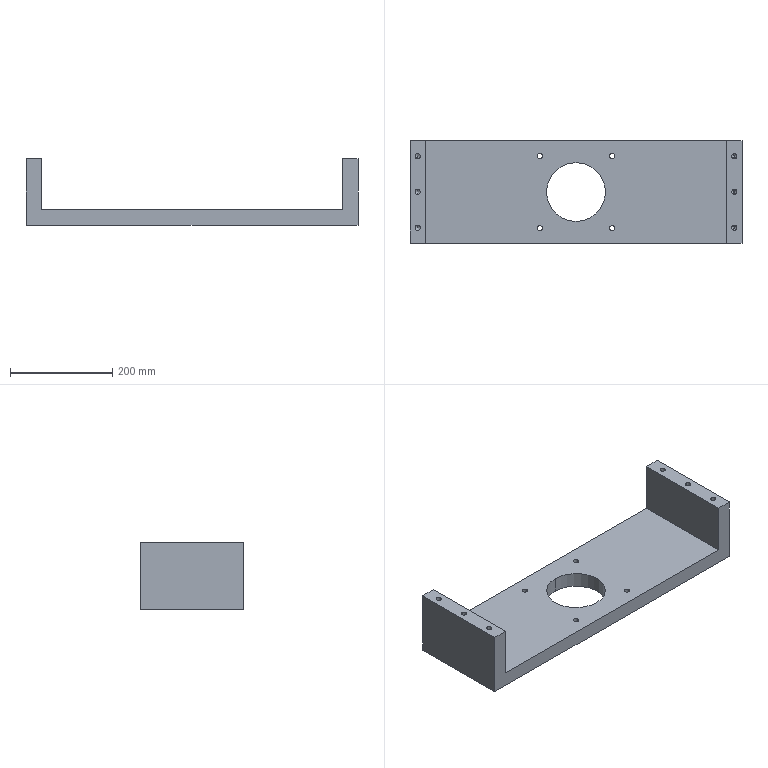Part | SolidWorks | features 3DProfileFeature 1, BaseBody 1, HoleWzd 1, SketchPattern 1 | 1 solid | 44 faces | box 650 x 200 x 130 mm | volume 4762030 mm3 | cylinder 22 | cone 12 | plane 10 | commonest cylinder face diameters 10.2 x20 115 x2
STEP:
#1=CARTESIAN_POINT('',(-65.611,-70.711,15.));
#2=VERTEX_POINT('',#1);
#3=CARTESIAN_POINT('',(-75.811,-70.711,15.));
#4=VERTEX_POINT('',#3);
#5=CARTESIAN_POINT('',(-70.711,-70.711,15.));
#6=DIRECTION('',(0.,0.,-1.));
#7=DIRECTION('',(-1.,0.,0.));
#8=AXIS2_PLACEMENT_3D('',#5,#6,#7);
#9=CIRCLE('',#8,5.1);
#10=EDGE_CURVE('',#2,#4,#9,.T.);
#11=ORIENTED_EDGE('',*,*,#10,.F.);
#12=CARTESIAN_POINT('',(-65.611,-70.711,-15.));
#13=VERTEX_POINT('',#12);
#14=CARTESIAN_POINT('',(-65.611,-70.711,-15.));
#15=DIRECTION('',(0.,0.,-1.));
#16=VECTOR('',#15,1000.);
#17=LINE('',#14,#16);
#18=EDGE_CURVE('',#2,#13,#17,.T.);
#19=ORIENTED_EDGE('',*,*,#18,.T.);
#20=CARTESIAN_POINT('',(-75.811,-70.711,-15.));
#21=VERTEX_POINT('',#20);
#22=CARTESIAN_POINT('',(-70.711,-70.711,-15.));
#23=DIRECTION('',(0.,0.,-1.));
#24=DIRECTION('',(-1.,0.,0.));
#25=AXIS2_PLACEMENT_3D('',#22,#23,#24);
#26=CIRCLE('',#25,5.1);
#27=EDGE_CURVE('',#13,#21,#26,.T.);
#28=ORIENTED_EDGE('',*,*,#27,.T.);
#29=CARTESIAN_POINT('',(-75.811,-70.711,-15.));
#30=DIRECTION('',(0.,0.,-1.));
#31=VECTOR('',#30,1000.);
#32=LINE('',#29,#31);
#33=EDGE_CURVE('',#4,#21,#32,.T.);
#34=ORIENTED_EDGE('',*,*,#33,.F.);
#35=EDGE_LOOP('',(#11,#19,#28,#34));
#36=FACE_OUTER_BOUND('',#35,.T.);
#37=CARTESIAN_POINT('',(-70.711,-70.711,-15.));
#38=DIRECTION('',(0.,0.,-1.));
#39=DIRECTION('',(-1.,0.,0.));
#40=AXIS2_PLACEMENT_3D('',#37,#38,#39);
#41=CYLINDRICAL_SURFACE('',#40,5.1);
#42=ADVANCED_FACE('',(#36),#41,.F.);
#43=CARTESIAN_POINT('',(75.811,-70.711,15.));
#44=VERTEX_POINT('',#43);
#45=CARTESIAN_POINT('',(65.611,-70.711,15.));
#46=VERTEX_POINT('',#45);
#47=CARTESIAN_POINT('',(70.711,-70.711,15.));
#48=DIRECTION('',(0.,0.,-1.));
#49=DIRECTION('',(-1.,0.,0.));
#50=AXIS2_PLACEMENT_3D('',#47,#48,#49);
#51=CIRCLE('',#50,5.1);
#52=EDGE_CURVE('',#44,#46,#51,.T.);
#53=ORIENTED_EDGE('',*,*,#52,.F.);
#54=CARTESIAN_POINT('',(75.811,-70.711,-15.));
#55=VERTEX_POINT('',#54);
#56=CARTESIAN_POINT('',(75.811,-70.711,-15.));
#57=DIRECTION('',(0.,0.,-1.));
#58=VECTOR('',#57,1000.);
#59=LINE('',#56,#58);
#60=EDGE_CURVE('',#44,#55,#59,.T.);
#61=ORIENTED_EDGE('',*,*,#60,.T.);
#62=CARTESIAN_POINT('',(65.611,-70.711,-15.));
#63=VERTEX_POINT('',#62);
#64=CARTESIAN_POINT('',(70.711,-70.711,-15.));
#65=DIRECTION('',(0.,0.,-1.));
#66=DIRECTION('',(-1.,0.,0.));
#67=AXIS2_PLACEMENT_3D('',#64,#65,#66);
#68=CIRCLE('',#67,5.1);
#69=EDGE_CURVE('',#55,#63,#68,.T.);
#70=ORIENTED_EDGE('',*,*,#69,.T.);
#71=CARTESIAN_POINT('',(65.611,-70.711,-15.));
#72=DIRECTION('',(0.,0.,-1.));
#73=VECTOR('',#72,1000.);
#74=LINE('',#71,#73);
#75=EDGE_CURVE('',#46,#63,#74,.T.);
#76=ORIENTED_EDGE('',*,*,#75,.F.);
#77=EDGE_LOOP('',(#53,#61,#70,#76));
#78=FACE_OUTER_BOUND('',#77,.T.);
#79=CARTESIAN_POINT('',(70.711,-70.711,-15.));
#80=DIRECTION('',(0.,0.,-1.));
#81=DIRECTION('',(-1.,0.,0.));
#82=AXIS2_PLACEMENT_3D('',#79,#80,#81);
#83=CYLINDRICAL_SURFACE('',#82,5.1);
#84=ADVANCED_FACE('',(#78),#83,.F.);
#85=CARTESIAN_POINT('',(75.811,70.711,15.));
#86=VERTEX_POINT('',#85);
#87=CARTESIAN_POINT('',(65.611,70.711,15.));
#88=VERTEX_POINT('',#87);
#89=CARTESIAN_POINT('',(70.711,70.711,15.));
#90=DIRECTION('',(0.,0.,-1.));
#91=DIRECTION('',(-1.,0.,0.));
#92=AXIS2_PLACEMENT_3D('',#89,#90,#91);
#93=CIRCLE('',#92,5.1);
#94=EDGE_CURVE('',#86,#88,#93,.T.);
#95=ORIENTED_EDGE('',*,*,#94,.F.);
#96=CARTESIAN_POINT('',(75.811,70.711,-15.));
#97=VERTEX_POINT('',#96);
#98=CARTESIAN_POINT('',(75.811,70.711,-15.));
#99=DIRECTION('',(0.,0.,-1.));
#100=VECTOR('',#99,1000.);
#101=LINE('',#98,#100);
#102=EDGE_CURVE('',#86,#97,#101,.T.);
#103=ORIENTED_EDGE('',*,*,#102,.T.);
#104=CARTESIAN_POINT('',(65.611,70.711,-15.));
#105=VERTEX_POINT('',#104);
#106=CARTESIAN_POINT('',(70.711,70.711,-15.));
#107=DIRECTION('',(0.,0.,-1.));
#108=DIRECTION('',(-1.,0.,0.));
#109=AXIS2_PLACEMENT_3D('',#106,#107,#108);
#110=CIRCLE('',#109,5.1);
#111=EDGE_CURVE('',#97,#105,#110,.T.);
#112=ORIENTED_EDGE('',*,*,#111,.T.);
#113=CARTESIAN_POINT('',(65.611,70.711,-15.));
#114=DIRECTION('',(0.,0.,-1.));
#115=VECTOR('',#114,1000.);
#116=LINE('',#113,#115);
#117=EDGE_CURVE('',#88,#105,#116,.T.);
#118=ORIENTED_EDGE('',*,*,#117,.F.);
#119=EDGE_LOOP('',(#95,#103,#112,#118));
#120=FACE_OUTER_BOUND('',#119,.T.);
#121=CARTESIAN_POINT('',(70.711,70.711,-15.));
#122=DIRECTION('',(0.,0.,-1.));
#123=DIRECTION('',(-1.,0.,0.));
#124=AXIS2_PLACEMENT_3D('',#121,#122,#123);
#125=CYLINDRICAL_SURFACE('',#124,5.1);
#126=ADVANCED_FACE('',(#120),#125,.F.);
#127=CARTESIAN_POINT('',(-65.611,70.711,15.));
#128=VERTEX_POINT('',#127);
#129=CARTESIAN_POINT('',(-75.811,70.711,15.));
#130=VERTEX_POINT('',#129);
#131=CARTESIAN_POINT('',(-70.711,70.711,15.));
#132=DIRECTION('',(0.,0.,-1.));
#133=DIRECTION('',(-1.,0.,0.));
#134=AXIS2_PLACEMENT_3D('',#131,#132,#133);
#135=CIRCLE('',#134,5.1);
#136=EDGE_CURVE('',#128,#130,#135,.T.);
#137=ORIENTED_EDGE('',*,*,#136,.F.);
#138=CARTESIAN_POINT('',(-65.611,70.711,-15.));
#139=VERTEX_POINT('',#138);
#140=CARTESIAN_POINT('',(-65.611,70.711,-15.));
#141=DIRECTION('',(0.,0.,-1.));
#142=VECTOR('',#141,1000.);
#143=LINE('',#140,#142);
#144=EDGE_CURVE('',#128,#139,#143,.T.);
#145=ORIENTED_EDGE('',*,*,#144,.T.);
#146=CARTESIAN_POINT('',(-75.811,70.711,-15.));
#147=VERTEX_POINT('',#146);
#148=CARTESIAN_POINT('',(-70.711,70.711,-15.));
#149=DIRECTION('',(0.,0.,-1.));
#150=DIRECTION('',(-1.,0.,0.));
#151=AXIS2_PLACEMENT_3D('',#148,#149,#150);
#152=CIRCLE('',#151,5.1);
#153=EDGE_CURVE('',#139,#147,#152,.T.);
#154=ORIENTED_EDGE('',*,*,#153,.T.);
#155=CARTESIAN_POINT('',(-75.811,70.711,-15.));
#156=DIRECTION('',(0.,0.,-1.));
#157=VECTOR('',#156,1000.);
#158=LINE('',#155,#157);
#159=EDGE_CURVE('',#130,#147,#158,.T.);
#160=ORIENTED_EDGE('',*,*,#159,.F.);
#161=EDGE_LOOP('',(#137,#145,#154,#160));
#162=FACE_OUTER_BOUND('',#161,.T.);
#163=CARTESIAN_POINT('',(-70.711,70.711,-15.));
#164=DIRECTION('',(0.,0.,-1.));
#165=DIRECTION('',(-1.,0.,0.));
#166=AXIS2_PLACEMENT_3D('',#163,#164,#165);
#167=CYLINDRICAL_SURFACE('',#166,5.1);
#168=ADVANCED_FACE('',(#162),#167,.F.);
#169=CARTESIAN_POINT('',(-310.,64.9,82.25));
#170=VERTEX_POINT('',#169);
#171=CARTESIAN_POINT('',(-310.,75.1,82.25));
#172=VERTEX_POINT('',#171);
#173=CARTESIAN_POINT('',(-310.,70.,82.25));
#174=DIRECTION('',(0.,0.,-1.));
#175=DIRECTION('',(1.,0.,0.));
#176=AXIS2_PLACEMENT_3D('',#173,#174,#175);
#177=CIRCLE('',#176,5.1);
#178=EDGE_CURVE('',#170,#172,#177,.T.);
#179=ORIENTED_EDGE('',*,*,#178,.T.);
#180=CARTESIAN_POINT('',(-310.,75.1,115.));
#181=VERTEX_POINT('',#180);
#182=CARTESIAN_POINT('',(-310.,75.1,82.25));
#183=DIRECTION('',(0.,0.,1.));
#184=VECTOR('',#183,1000.);
#185=LINE('',#182,#184);
#186=EDGE_CURVE('',#172,#181,#185,.T.);
#187=ORIENTED_EDGE('',*,*,#186,.T.);
#188=CARTESIAN_POINT('',(-310.,64.9,115.));
#189=VERTEX_POINT('',#188);
#190=CARTESIAN_POINT('',(-310.,70.,115.));
#191=DIRECTION('',(0.,0.,1.));
#192=DIRECTION('',(0.,-1.,0.));
#193=AXIS2_PLACEMENT_3D('',#190,#191,#192);
#194=CIRCLE('',#193,5.1);
#195=EDGE_CURVE('',#181,#189,#194,.T.);
#196=ORIENTED_EDGE('',*,*,#195,.T.);
#197=CARTESIAN_POINT('',(-310.,64.9,82.25));
#198=DIRECTION('',(0.,0.,1.));
#199=VECTOR('',#198,1000.);
#200=LINE('',#197,#199);
#201=EDGE_CURVE('',#170,#189,#200,.T.);
#202=ORIENTED_EDGE('',*,*,#201,.F.);
#203=EDGE_LOOP('',(#179,#187,#196,#202));
#204=FACE_OUTER_BOUND('',#203,.T.);
#205=CARTESIAN_POINT('',(-310.,70.,82.25));
#206=DIRECTION('',(0.,0.,1.));
#207=DIRECTION('',(0.,-1.,0.));
#208=AXIS2_PLACEMENT_3D('',#205,#206,#207);
#209=CYLINDRICAL_SURFACE('',#208,5.1);
#210=ADVANCED_FACE('',(#204),#209,.F.);
#211=CARTESIAN_POINT('',(-310.,70.,79.186));
#212=VERTEX_POINT('',#211);
#213=CARTESIAN_POINT('',(-310.,70.,79.186));
#214=DIRECTION('',(0.,-0.8572,0.515));
#215=VECTOR('',#214,1000.);
#216=LINE('',#213,#215);
#217=EDGE_CURVE('',#212,#170,#216,.T.);
#218=ORIENTED_EDGE('',*,*,#217,.F.);
#219=CARTESIAN_POINT('',(-310.,70.,79.186));
#220=DIRECTION('',(0.,0.8572,0.515));
#221=VECTOR('',#220,1000.);
#222=LINE('',#219,#221);
#223=EDGE_CURVE('',#212,#172,#222,.T.);
#224=ORIENTED_EDGE('',*,*,#223,.T.);
#225=ORIENTED_EDGE('',*,*,#178,.F.);
#226=EDGE_LOOP('',(#218,#224,#225));
#227=FACE_OUTER_BOUND('',#226,.T.);
#228=CARTESIAN_POINT('',(-310.,70.,1079.186));
#229=DIRECTION('',(0.,0.,1.));
#230=DIRECTION('',(0.,-1.,0.));
#231=AXIS2_PLACEMENT_3D('',#228,#229,#230);
#232=CONICAL_SURFACE('',#231,1664.279,1.03);
#233=ADVANCED_FACE('',(#227),#232,.F.);
#234=CARTESIAN_POINT('',(-310.,-75.1,82.25));
#235=VERTEX_POINT('',#234);
#236=CARTESIAN_POINT('',(-310.,-64.9,82.25));
#237=VERTEX_POINT('',#236);
#238=CARTESIAN_POINT('',(-310.,-70.,82.25));
#239=DIRECTION('',(0.,0.,-1.));
#240=DIRECTION('',(1.,0.,0.));
#241=AXIS2_PLACEMENT_3D('',#238,#239,#240);
#242=CIRCLE('',#241,5.1);
#243=EDGE_CURVE('',#235,#237,#242,.T.);
#244=ORIENTED_EDGE('',*,*,#243,.T.);
#245=CARTESIAN_POINT('',(-310.,-64.9,115.));
#246=VERTEX_POINT('',#245);
#247=CARTESIAN_POINT('',(-310.,-64.9,82.25));
#248=DIRECTION('',(0.,0.,1.));
#249=VECTOR('',#248,1000.);
#250=LINE('',#247,#249);
#251=EDGE_CURVE('',#237,#246,#250,.T.);
#252=ORIENTED_EDGE('',*,*,#251,.T.);
#253=CARTESIAN_POINT('',(-310.,-75.1,115.));
#254=VERTEX_POINT('',#253);
#255=CARTESIAN_POINT('',(-310.,-70.,115.));
#256=DIRECTION('',(0.,0.,-1.));
#257=DIRECTION('',(0.,-1.,0.));
#258=AXIS2_PLACEMENT_3D('',#255,#256,#257);
#259=CIRCLE('',#258,5.1);
#260=EDGE_CURVE('',#254,#246,#259,.T.);
#261=ORIENTED_EDGE('',*,*,#260,.F.);
#262=CARTESIAN_POINT('',(-310.,-75.1,82.25));
#263=DIRECTION('',(0.,0.,1.));
#264=VECTOR('',#263,1000.);
#265=LINE('',#262,#264);
#266=EDGE_CURVE('',#235,#254,#265,.T.);
#267=ORIENTED_EDGE('',*,*,#266,.F.);
#268=EDGE_LOOP('',(#244,#252,#261,#267));
#269=FACE_OUTER_BOUND('',#268,.T.);
#270=CARTESIAN_POINT('',(-310.,-70.,82.25));
#271=DIRECTION('',(0.,0.,1.));
#272=DIRECTION('',(0.,-1.,0.));
#273=AXIS2_PLACEMENT_3D('',#270,#271,#272);
#274=CYLINDRICAL_SURFACE('',#273,5.1);
#275=ADVANCED_FACE('',(#269),#274,.F.);
#276=CARTESIAN_POINT('',(-310.,-5.1,82.25));
#277=VERTEX_POINT('',#276);
#278=CARTESIAN_POINT('',(-310.,5.1,82.25));
#279=VERTEX_POINT('',#278);
#280=CARTESIAN_POINT('',(-310.,0.,82.25));
#281=DIRECTION('',(0.,0.,-1.));
#282=DIRECTION('',(1.,0.,0.));
#283=AXIS2_PLACEMENT_3D('',#280,#281,#282);
#284=CIRCLE('',#283,5.1);
#285=EDGE_CURVE('',#277,#279,#284,.T.);
#286=ORIENTED_EDGE('',*,*,#285,.T.);
#287=CARTESIAN_POINT('',(-310.,5.1,115.));
#288=VERTEX_POINT('',#287);
#289=CARTESIAN_POINT('',(-310.,5.1,82.25));
#290=DIRECTION('',(0.,0.,1.));
#291=VECTOR('',#290,1000.);
#292=LINE('',#289,#291);
#293=EDGE_CURVE('',#279,#288,#292,.T.);
#294=ORIENTED_EDGE('',*,*,#293,.T.);
#295=CARTESIAN_POINT('',(-310.,-5.1,115.));
#296=VERTEX_POINT('',#295);
#297=CARTESIAN_POINT('',(-310.,0.,115.));
#298=DIRECTION('',(0.,0.,-1.));
#299=DIRECTION('',(0.,-1.,0.));
#300=AXIS2_PLACEMENT_3D('',#297,#298,#299);
#301=CIRCLE('',#300,5.1);
#302=EDGE_CURVE('',#296,#288,#301,.T.);
#303=ORIENTED_EDGE('',*,*,#302,.F.);
#304=CARTESIAN_POINT('',(-310.,-5.1,82.25));
#305=DIRECTION('',(0.,0.,1.));
#306=VECTOR('',#305,1000.);
#307=LINE('',#304,#306);
#308=EDGE_CURVE('',#277,#296,#307,.T.);
#309=ORIENTED_EDGE('',*,*,#308,.F.);
#310=EDGE_LOOP('',(#286,#294,#303,#309));
#311=FACE_OUTER_BOUND('',#310,.T.);
#312=CARTESIAN_POINT('',(-310.,0.,82.25));
#313=DIRECTION('',(0.,0.,1.));
#314=DIRECTION('',(0.,-1.,0.));
#315=AXIS2_PLACEMENT_3D('',#312,#313,#314);
#316=CYLINDRICAL_SURFACE('',#315,5.1);
#317=ADVANCED_FACE('',(#311),#316,.F.);
#318=CARTESIAN_POINT('',(-310.,-70.,79.186));
#319=VERTEX_POINT('',#318);
#320=CARTESIAN_POINT('',(-310.,-70.,79.186));
#321=DIRECTION('',(0.,-0.8572,0.515));
#322=VECTOR('',#321,1000.);
#323=LINE('',#320,#322);
#324=EDGE_CURVE('',#319,#235,#323,.T.);
#325=ORIENTED_EDGE('',*,*,#324,.F.);
#326=CARTESIAN_POINT('',(-310.,-70.,79.186));
#327=DIRECTION('',(0.,0.8572,0.515));
#328=VECTOR('',#327,1000.);
#329=LINE('',#326,#328);
#330=EDGE_CURVE('',#319,#237,#329,.T.);
#331=ORIENTED_EDGE('',*,*,#330,.T.);
#332=ORIENTED_EDGE('',*,*,#243,.F.);
#333=EDGE_LOOP('',(#325,#331,#332));
#334=FACE_OUTER_BOUND('',#333,.T.);
#335=CARTESIAN_POINT('',(-310.,-70.,1079.186));
#336=DIRECTION('',(0.,0.,1.));
#337=DIRECTION('',(0.,-1.,0.));
#338=AXIS2_PLACEMENT_3D('',#335,#336,#337);
#339=CONICAL_SURFACE('',#338,1664.279,1.03);
#340=ADVANCED_FACE('',(#334),#339,.F.);
#341=CARTESIAN_POINT('',(-310.,0.,79.186));
#342=VERTEX_POINT('',#341);
#343=CARTESIAN_POINT('',(-310.,0.,79.186));
#344=DIRECTION('',(0.,-0.8572,0.515));
#345=VECTOR('',#344,1000.);
#346=LINE('',#343,#345);
#347=EDGE_CURVE('',#342,#277,#346,.T.);
#348=ORIENTED_EDGE('',*,*,#347,.F.);
#349=CARTESIAN_POINT('',(-310.,0.,79.186));
#350=DIRECTION('',(0.,0.8572,0.515));
#351=VECTOR('',#350,1000.);
#352=LINE('',#349,#351);
#353=EDGE_CURVE('',#342,#279,#352,.T.);
#354=ORIENTED_EDGE('',*,*,#353,.T.);
#355=ORIENTED_EDGE('',*,*,#285,.F.);
#356=EDGE_LOOP('',(#348,#354,#355));
#357=FACE_OUTER_BOUND('',#356,.T.);
#358=CARTESIAN_POINT('',(-310.,0.,1079.186));
#359=DIRECTION('',(0.,0.,1.));
#360=DIRECTION('',(0.,-1.,0.));
#361=AXIS2_PLACEMENT_3D('',#358,#359,#360);
#362=CONICAL_SURFACE('',#361,1664.279,1.03);
#363=ADVANCED_FACE('',(#357),#362,.F.);
#364=CARTESIAN_POINT('',(0.,57.5,-15.));
#365=VERTEX_POINT('',#364);
#366=CARTESIAN_POINT('',(0.,-57.5,-15.));
#367=VERTEX_POINT('',#366);
#368=CARTESIAN_POINT('',(0.,0.,-15.));
#369=DIRECTION('',(0.,0.,1.));
#370=DIRECTION('',(0.,-1.,0.));
#371=AXIS2_PLACEMENT_3D('',#368,#369,#370);
#372=CIRCLE('',#371,57.5);
#373=EDGE_CURVE('',#365,#367,#372,.T.);
#374=ORIENTED_EDGE('',*,*,#373,.F.);
#375=CARTESIAN_POINT('',(0.,57.5,15.));
#376=VERTEX_POINT('',#375);
#377=CARTESIAN_POINT('',(0.,57.5,-15.));
#378=DIRECTION('',(0.,0.,1.));
#379=VECTOR('',#378,1000.);
#380=LINE('',#377,#379);
#381=EDGE_CURVE('',#365,#376,#380,.T.);
#382=ORIENTED_EDGE('',*,*,#381,.T.);
#383=CARTESIAN_POINT('',(0.,-57.5,15.));
#384=VERTEX_POINT('',#383);
#385=CARTESIAN_POINT('',(0.,0.,15.));
#386=DIRECTION('',(0.,0.,1.));
#387=DIRECTION('',(0.,-1.,0.));
#388=AXIS2_PLACEMENT_3D('',#385,#386,#387);
#389=CIRCLE('',#388,57.5);
#390=EDGE_CURVE('',#376,#384,#389,.T.);
#391=ORIENTED_EDGE('',*,*,#390,.T.);
#392=CARTESIAN_POINT('',(0.,-57.5,-15.));
#393=DIRECTION('',(0.,0.,1.));
#394=VECTOR('',#393,1000.);
#395=LINE('',#392,#394);
#396=EDGE_CURVE('',#367,#384,#395,.T.);
#397=ORIENTED_EDGE('',*,*,#396,.F.);
#398=EDGE_LOOP('',(#374,#382,#391,#397));
#399=FACE_OUTER_BOUND('',#398,.T.);
#400=CARTESIAN_POINT('',(0.,0.,-15.));
#401=DIRECTION('',(0.,0.,1.));
#402=DIRECTION('',(0.,-1.,0.));
#403=AXIS2_PLACEMENT_3D('',#400,#401,#402);
#404=CYLINDRICAL_SURFACE('',#403,57.5);
#405=ADVANCED_FACE('',(#399),#404,.F.);
#406=CARTESIAN_POINT('',(310.,64.9,82.25));
#407=VERTEX_POINT('',#406);
#408=CARTESIAN_POINT('',(310.,75.1,82.25));
#409=VERTEX_POINT('',#408);
#410=CARTESIAN_POINT('',(310.,70.,82.25));
#411=DIRECTION('',(0.,0.,-1.));
#412=DIRECTION('',(1.,0.,0.));
#413=AXIS2_PLACEMENT_3D('',#410,#411,#412);
#414=CIRCLE('',#413,5.1);
#415=EDGE_CURVE('',#407,#409,#414,.T.);
#416=ORIENTED_EDGE('',*,*,#415,.T.);
#417=CARTESIAN_POINT('',(310.,75.1,115.));
#418=VERTEX_POINT('',#417);
#419=CARTESIAN_POINT('',(310.,75.1,82.25));
#420=DIRECTION('',(0.,0.,1.));
#421=VECTOR('',#420,1000.);
#422=LINE('',#419,#421);
#423=EDGE_CURVE('',#409,#418,#422,.T.);
#424=ORIENTED_EDGE('',*,*,#423,.T.);
#425=CARTESIAN_POINT('',(310.,64.9,115.));
#426=VERTEX_POINT('',#425);
#427=CARTESIAN_POINT('',(310.,70.,115.));
#428=DIRECTION('',(0.,0.,-1.));
#429=DIRECTION('',(0.,-1.,0.));
#430=AXIS2_PLACEMENT_3D('',#427,#428,#429);
#431=CIRCLE('',#430,5.1);
#432=EDGE_CURVE('',#426,#418,#431,.T.);
#433=ORIENTED_EDGE('',*,*,#432,.F.);
#434=CARTESIAN_POINT('',(310.,64.9,82.25));
#435=DIRECTION('',(0.,0.,1.));
#436=VECTOR('',#435,1000.);
#437=LINE('',#434,#436);
#438=EDGE_CURVE('',#407,#426,#437,.T.);
#439=ORIENTED_EDGE('',*,*,#438,.F.);
#440=EDGE_LOOP('',(#416,#424,#433,#439));
#441=FACE_OUTER_BOUND('',#440,.T.);
#442=CARTESIAN_POINT('',(310.,70.,82.25));
#443=DIRECTION('',(0.,0.,1.));
#444=DIRECTION('',(0.,-1.,0.));
#445=AXIS2_PLACEMENT_3D('',#442,#443,#444);
#446=CYLINDRICAL_SURFACE('',#445,5.1);
#447=ADVANCED_FACE('',(#441),#446,.F.);
#448=CARTESIAN_POINT('',(310.,-5.1,82.25));
#449=VERTEX_POINT('',#448);
#450=CARTESIAN_POINT('',(310.,5.1,82.25));
#451=VERTEX_POINT('',#450);
#452=CARTESIAN_POINT('',(310.,0.,82.25));
#453=DIRECTION('',(0.,0.,-1.));
#454=DIRECTION('',(1.,0.,0.));
#455=AXIS2_PLACEMENT_3D('',#452,#453,#454);
#456=CIRCLE('',#455,5.1);
#457=EDGE_CURVE('',#449,#451,#456,.T.);
#458=ORIENTED_EDGE('',*,*,#457,.T.);
#459=CARTESIAN_POINT('',(310.,5.1,115.));
#460=VERTEX_POINT('',#459);
#461=CARTESIAN_POINT('',(310.,5.1,82.25));
#462=DIRECTION('',(0.,0.,1.));
#463=VECTOR('',#462,1000.);
#464=LINE('',#461,#463);
#465=EDGE_CURVE('',#451,#460,#464,.T.);
#466=ORIENTED_EDGE('',*,*,#465,.T.);
#467=CARTESIAN_POINT('',(310.,-5.1,115.));
#468=VERTEX_POINT('',#467);
#469=CARTESIAN_POINT('',(310.,0.,115.));
#470=DIRECTION('',(0.,0.,-1.));
#471=DIRECTION('',(0.,-1.,0.));
#472=AXIS2_PLACEMENT_3D('',#469,#470,#471);
#473=CIRCLE('',#472,5.1);
#474=EDGE_CURVE('',#468,#460,#473,.T.);
#475=ORIENTED_EDGE('',*,*,#474,.F.);
#476=CARTESIAN_POINT('',(310.,-5.1,82.25));
#477=DIRECTION('',(0.,0.,1.));
#478=VECTOR('',#477,1000.);
#479=LINE('',#476,#478);
#480=EDGE_CURVE('',#449,#468,#479,.T.);
#481=ORIENTED_EDGE('',*,*,#480,.F.);
#482=EDGE_LOOP('',(#458,#466,#475,#481));
#483=FACE_OUTER_BOUND('',#482,.T.);
#484=CARTESIAN_POINT('',(310.,0.,82.25));
#485=DIRECTION('',(0.,0.,1.));
#486=DIRECTION('',(0.,-1.,0.));
#487=AXIS2_PLACEMENT_3D('',#484,#485,#486);
#488=CYLINDRICAL_SURFACE('',#487,5.1);
#489=ADVANCED_FACE('',(#483),#488,.F.);
#490=CARTESIAN_POINT('',(310.,-75.1,82.25));
#491=VERTEX_POINT('',#490);
#492=CARTESIAN_POINT('',(310.,-64.9,82.25));
#493=VERTEX_POINT('',#492);
#494=CARTESIAN_POINT('',(310.,-70.,82.25));
#495=DIRECTION('',(0.,0.,-1.));
#496=DIRECTION('',(1.,0.,0.));
#497=AXIS2_PLACEMENT_3D('',#494,#495,#496);
#498=CIRCLE('',#497,5.1);
#499=EDGE_CURVE('',#491,#493,#498,.T.);
#500=ORIENTED_EDGE('',*,*,#499,.T.);
#501=CARTESIAN_POINT('',(310.,-64.9,115.));
#502=VERTEX_POINT('',#501);
#503=CARTESIAN_POINT('',(310.,-64.9,82.25));
#504=DIRECTION('',(0.,0.,1.));
#505=VECTOR('',#504,1000.);
#506=LINE('',#503,#505);
#507=EDGE_CURVE('',#493,#502,#506,.T.);
#508=ORIENTED_EDGE('',*,*,#507,.T.);
#509=CARTESIAN_POINT('',(310.,-75.1,115.));
#510=VERTEX_POINT('',#509);
#511=CARTESIAN_POINT('',(310.,-70.,115.));
#512=DIRECTION('',(0.,0.,-1.));
#513=DIRECTION('',(0.,-1.,0.));
#514=AXIS2_PLACEMENT_3D('',#511,#512,#513);
#515=CIRCLE('',#514,5.1);
#516=EDGE_CURVE('',#510,#502,#515,.T.);
#517=ORIENTED_EDGE('',*,*,#516,.F.);
#518=CARTESIAN_POINT('',(310.,-75.1,82.25));
#519=DIRECTION('',(0.,0.,1.));
#520=VECTOR('',#519,1000.);
#521=LINE('',#518,#520);
#522=EDGE_CURVE('',#491,#510,#521,.T.);
#523=ORIENTED_EDGE('',*,*,#522,.F.);
#524=EDGE_LOOP('',(#500,#508,#517,#523));
#525=FACE_OUTER_BOUND('',#524,.T.);
#526=CARTESIAN_POINT('',(310.,-70.,82.25));
#527=DIRECTION('',(0.,0.,1.));
#528=DIRECTION('',(0.,-1.,0.));
#529=AXIS2_PLACEMENT_3D('',#526,#527,#528);
#530=CYLINDRICAL_SURFACE('',#529,5.1);
#531=ADVANCED_FACE('',(#525),#530,.F.);
#532=CARTESIAN_POINT('',(310.,70.,79.186));
#533=VERTEX_POINT('',#532);
#534=CARTESIAN_POINT('',(310.,70.,79.186));
#535=DIRECTION('',(0.,-0.8572,0.515));
#536=VECTOR('',#535,1000.);
#537=LINE('',#534,#536);
#538=EDGE_CURVE('',#533,#407,#537,.T.);
#539=ORIENTED_EDGE('',*,*,#538,.F.);
#540=CARTESIAN_POINT('',(310.,70.,79.186));
#541=DIRECTION('',(0.,0.8572,0.515));
#542=VECTOR('',#541,1000.);
#543=LINE('',#540,#542);
#544=EDGE_CURVE('',#533,#409,#543,.T.);
#545=ORIENTED_EDGE('',*,*,#544,.T.);
#546=ORIENTED_EDGE('',*,*,#415,.F.);
#547=EDGE_LOOP('',(#539,#545,#546));
#548=FACE_OUTER_BOUND('',#547,.T.);
#549=CARTESIAN_POINT('',(310.,70.,1079.186));
#550=DIRECTION('',(0.,0.,1.));
#551=DIRECTION('',(0.,-1.,0.));
#552=AXIS2_PLACEMENT_3D('',#549,#550,#551);
#553=CONICAL_SURFACE('',#552,1664.279,1.03);
#554=ADVANCED_FACE('',(#548),#553,.F.);
#555=CARTESIAN_POINT('',(310.,0.,79.186));
#556=VERTEX_POINT('',#555);
#557=CARTESIAN_POINT('',(310.,0.,79.186));
#558=DIRECTION('',(0.,-0.8572,0.515));
#559=VECTOR('',#558,1000.);
#560=LINE('',#557,#559);
#561=EDGE_CURVE('',#556,#449,#560,.T.);
#562=ORIENTED_EDGE('',*,*,#561,.F.);
#563=CARTESIAN_POINT('',(310.,0.,79.186));
#564=DIRECTION('',(0.,0.8572,0.515));
#565=VECTOR('',#564,1000.);
#566=LINE('',#563,#565);
#567=EDGE_CURVE('',#556,#451,#566,.T.);
#568=ORIENTED_EDGE('',*,*,#567,.T.);
#569=ORIENTED_EDGE('',*,*,#457,.F.);
#570=EDGE_LOOP('',(#562,#568,#569));
#571=FACE_OUTER_BOUND('',#570,.T.);
#572=CARTESIAN_POINT('',(310.,0.,1079.186));
#573=DIRECTION('',(0.,0.,1.));
#574=DIRECTION('',(0.,-1.,0.));
#575=AXIS2_PLACEMENT_3D('',#572,#573,#574);
#576=CONICAL_SURFACE('',#575,1664.279,1.03);
#577=ADVANCED_FACE('',(#571),#576,.F.);
#578=CARTESIAN_POINT('',(310.,-70.,79.186));
#579=VERTEX_POINT('',#578);
#580=CARTESIAN_POINT('',(310.,-70.,79.186));
#581=DIRECTION('',(0.,-0.8572,0.515));
#582=VECTOR('',#581,1000.);
#583=LINE('',#580,#582);
#584=EDGE_CURVE('',#579,#491,#583,.T.);
#585=ORIENTED_EDGE('',*,*,#584,.F.);
#586=CARTESIAN_POINT('',(310.,-70.,79.186));
#587=DIRECTION('',(0.,0.8572,0.515));
#588=VECTOR('',#587,1000.);
#589=LINE('',#586,#588);
#590=EDGE_CURVE('',#579,#493,#589,.T.);
#591=ORIENTED_EDGE('',*,*,#590,.T.);
#592=ORIENTED_EDGE('',*,*,#499,.F.);
#593=EDGE_LOOP('',(#585,#591,#592));
#594=FACE_OUTER_BOUND('',#593,.T.);
#595=CARTESIAN_POINT('',(310.,-70.,1079.186));
#596=DIRECTION('',(0.,0.,1.));
#597=DIRECTION('',(0.,-1.,0.));
#598=AXIS2_PLACEMENT_3D('',#595,#596,#597);
#599=CONICAL_SURFACE('',#598,1664.279,1.03);
#600=ADVANCED_FACE('',(#594),#599,.F.);
#601=ORIENTED_EDGE('',*,*,#186,.F.);
#602=CARTESIAN_POINT('',(-310.,70.,82.25));
#603=DIRECTION('',(0.,0.,-1.));
#604=DIRECTION('',(1.,0.,0.));
#605=AXIS2_PLACEMENT_3D('',#602,#603,#604);
#606=CIRCLE('',#605,5.1);
#607=EDGE_CURVE('',#172,#170,#606,.T.);
#608=ORIENTED_EDGE('',*,*,#607,.T.);
#609=ORIENTED_EDGE('',*,*,#201,.T.);
#610=CARTESIAN_POINT('',(-310.,70.,115.));
#611=DIRECTION('',(0.,0.,1.));
#612=DIRECTION('',(0.,-1.,0.));
#613=AXIS2_PLACEMENT_3D('',#610,#611,#612);
#614=CIRCLE('',#613,5.1);
#615=EDGE_CURVE('',#189,#181,#614,.T.);
#616=ORIENTED_EDGE('',*,*,#615,.T.);
#617=EDGE_LOOP('',(#601,#608,#609,#616));
#618=FACE_OUTER_BOUND('',#617,.T.);
#619=CARTESIAN_POINT('',(-310.,70.,82.25));
#620=DIRECTION('',(0.,0.,1.));
#621=DIRECTION('',(0.,-1.,0.));
#622=AXIS2_PLACEMENT_3D('',#619,#620,#621);
#623=CYLINDRICAL_SURFACE('',#622,5.1);
#624=ADVANCED_FACE('',(#618),#623,.F.);
#625=ORIENTED_EDGE('',*,*,#260,.T.);
#626=CARTESIAN_POINT('',(-310.,-70.,115.));
#627=DIRECTION('',(0.,0.,-1.));
#628=DIRECTION('',(0.,-1.,0.));
#629=AXIS2_PLACEMENT_3D('',#626,#627,#628);
#630=CIRCLE('',#629,5.1);
#631=EDGE_CURVE('',#246,#254,#630,.T.);
#632=ORIENTED_EDGE('',*,*,#631,.T.);
#633=EDGE_LOOP('',(#625,#632));
#634=FACE_BOUND('',#633,.T.);
#635=ORIENTED_EDGE('',*,*,#302,.T.);
#636=CARTESIAN_POINT('',(-310.,0.,115.));
#637=DIRECTION('',(0.,0.,-1.));
#638=DIRECTION('',(0.,-1.,0.));
#639=AXIS2_PLACEMENT_3D('',#636,#637,#638);
#640=CIRCLE('',#639,5.1);
#641=EDGE_CURVE('',#288,#296,#640,.T.);
#642=ORIENTED_EDGE('',*,*,#641,.T.);
#643=EDGE_LOOP('',(#635,#642));
#644=FACE_BOUND('',#643,.T.);
#645=ORIENTED_EDGE('',*,*,#615,.F.);
#646=ORIENTED_EDGE('',*,*,#195,.F.);
#647=EDGE_LOOP('',(#645,#646));
#648=FACE_BOUND('',#647,.T.);
#649=CARTESIAN_POINT('',(-295.,-100.,115.));
#650=VERTEX_POINT('',#649);
#651=CARTESIAN_POINT('',(-295.,100.,115.));
#652=VERTEX_POINT('',#651);
#653=CARTESIAN_POINT('',(-295.,0.,115.));
#654=DIRECTION('',(0.,1.,0.));
#655=VECTOR('',#654,1000.);
#656=LINE('',#653,#655);
#657=EDGE_CURVE('',#650,#652,#656,.T.);
#658=ORIENTED_EDGE('',*,*,#657,.T.);
#659=CARTESIAN_POINT('',(-325.,100.,115.));
#660=VERTEX_POINT('',#659);
#661=CARTESIAN_POINT('',(-310.,100.,115.));
#662=DIRECTION('',(-1.,0.,0.));
#663=VECTOR('',#662,1000.);
#664=LINE('',#661,#663);
#665=EDGE_CURVE('',#652,#660,#664,.T.);
#666=ORIENTED_EDGE('',*,*,#665,.T.);
#667=CARTESIAN_POINT('',(-325.,-100.,115.));
#668=VERTEX_POINT('',#667);
#669=CARTESIAN_POINT('',(-325.,0.,115.));
#670=DIRECTION('',(0.,-1.,0.));
#671=VECTOR('',#670,1000.);
#672=LINE('',#669,#671);
#673=EDGE_CURVE('',#660,#668,#672,.T.);
#674=ORIENTED_EDGE('',*,*,#673,.T.);
#675=CARTESIAN_POINT('',(-310.,-100.,115.));
#676=DIRECTION('',(1.,0.,0.));
#677=VECTOR('',#676,1000.);
#678=LINE('',#675,#677);
#679=EDGE_CURVE('',#668,#650,#678,.T.);
#680=ORIENTED_EDGE('',*,*,#679,.T.);
#681=EDGE_LOOP('',(#658,#666,#674,#680));
#682=FACE_OUTER_BOUND('',#681,.T.);
#683=CARTESIAN_POINT('',(-325.,-100.,115.));
#684=DIRECTION('',(0.,0.,1.));
#685=DIRECTION('',(1.,0.,0.));
#686=AXIS2_PLACEMENT_3D('',#683,#684,#685);
#687=PLANE('',#686);
#688=ADVANCED_FACE('',(#634,#644,#648,#682),#687,.T.);
#689=ORIENTED_EDGE('',*,*,#223,.F.);
#690=ORIENTED_EDGE('',*,*,#217,.T.);
#691=ORIENTED_EDGE('',*,*,#607,.F.);
#692=EDGE_LOOP('',(#689,#690,#691));
#693=FACE_OUTER_BOUND('',#692,.T.);
#694=CARTESIAN_POINT('',(-310.,70.,1079.186));
#695=DIRECTION('',(0.,0.,1.));
#696=DIRECTION('',(0.,-1.,0.));
#697=AXIS2_PLACEMENT_3D('',#694,#695,#696);
#698=CONICAL_SURFACE('',#697,1664.279,1.03);
#699=ADVANCED_FACE('',(#693),#698,.F.);
#700=ORIENTED_EDGE('',*,*,#251,.F.);
#701=CARTESIAN_POINT('',(-310.,-70.,82.25));
#702=DIRECTION('',(0.,0.,-1.));
#703=DIRECTION('',(1.,0.,0.));
#704=AXIS2_PLACEMENT_3D('',#701,#702,#703);
#705=CIRCLE('',#704,5.1);
#706=EDGE_CURVE('',#237,#235,#705,.T.);
#707=ORIENTED_EDGE('',*,*,#706,.T.);
#708=ORIENTED_EDGE('',*,*,#266,.T.);
#709=ORIENTED_EDGE('',*,*,#631,.F.);
#710=EDGE_LOOP('',(#700,#707,#708,#709));
#711=FACE_OUTER_BOUND('',#710,.T.);
#712=CARTESIAN_POINT('',(-310.,-70.,82.25));
#713=DIRECTION('',(0.,0.,1.));
#714=DIRECTION('',(0.,-1.,0.));
#715=AXIS2_PLACEMENT_3D('',#712,#713,#714);
#716=CYLINDRICAL_SURFACE('',#715,5.1);
#717=ADVANCED_FACE('',(#711),#716,.F.);
#718=ORIENTED_EDGE('',*,*,#293,.F.);
#719=CARTESIAN_POINT('',(-310.,0.,82.25));
#720=DIRECTION('',(0.,0.,-1.));
#721=DIRECTION('',(1.,0.,0.));
#722=AXIS2_PLACEMENT_3D('',#719,#720,#721);
#723=CIRCLE('',#722,5.1);
#724=EDGE_CURVE('',#279,#277,#723,.T.);
#725=ORIENTED_EDGE('',*,*,#724,.T.);
#726=ORIENTED_EDGE('',*,*,#308,.T.);
#727=ORIENTED_EDGE('',*,*,#641,.F.);
#728=EDGE_LOOP('',(#718,#725,#726,#727));
#729=FACE_OUTER_BOUND('',#728,.T.);
#730=CARTESIAN_POINT('',(-310.,0.,82.25));
#731=DIRECTION('',(0.,0.,1.));
#732=DIRECTION('',(0.,-1.,0.));
#733=AXIS2_PLACEMENT_3D('',#730,#731,#732);
#734=CYLINDRICAL_SURFACE('',#733,5.1);
#735=ADVANCED_FACE('',(#729),#734,.F.);
#736=CARTESIAN_POINT('',(-325.,100.,-15.));
#737=VERTEX_POINT('',#736);
#738=CARTESIAN_POINT('',(-325.,100.,50.));
#739=DIRECTION('',(0.,0.,-1.));
#740=VECTOR('',#739,1000.);
#741=LINE('',#738,#740);
#742=EDGE_CURVE('',#660,#737,#741,.T.);
#743=ORIENTED_EDGE('',*,*,#742,.F.);
#744=ORIENTED_EDGE('',*,*,#665,.F.);
#745=CARTESIAN_POINT('',(-295.,100.,15.));
#746=VERTEX_POINT('',#745);
#747=CARTESIAN_POINT('',(-295.,100.,50.));
#748=DIRECTION('',(0.,0.,1.));
#749=VECTOR('',#748,1000.);
#750=LINE('',#747,#749);
#751=EDGE_CURVE('',#746,#652,#750,.T.);
#752=ORIENTED_EDGE('',*,*,#751,.F.);
#753=CARTESIAN_POINT('',(295.,100.,15.));
#754=VERTEX_POINT('',#753);
#755=CARTESIAN_POINT('',(0.,100.,15.));
#756=DIRECTION('',(-1.,0.,0.));
#757=VECTOR('',#756,1000.);
#758=LINE('',#755,#757);
#759=EDGE_CURVE('',#754,#746,#758,.T.);
#760=ORIENTED_EDGE('',*,*,#759,.F.);
#761=CARTESIAN_POINT('',(295.,100.,115.));
#762=VERTEX_POINT('',#761);
#763=CARTESIAN_POINT('',(295.,100.,50.));
#764=DIRECTION('',(0.,0.,-1.));
#765=VECTOR('',#764,1000.);
#766=LINE('',#763,#765);
#767=EDGE_CURVE('',#762,#754,#766,.T.);
#768=ORIENTED_EDGE('',*,*,#767,.F.);
#769=CARTESIAN_POINT('',(325.,100.,115.));
#770=VERTEX_POINT('',#769);
#771=CARTESIAN_POINT('',(0.,100.,115.));
#772=DIRECTION('',(-1.,0.,0.));
#773=VECTOR('',#772,1000.);
#774=LINE('',#771,#773);
#775=EDGE_CURVE('',#770,#762,#774,.T.);
#776=ORIENTED_EDGE('',*,*,#775,.F.);
#777=CARTESIAN_POINT('',(325.,100.,-15.));
#778=VERTEX_POINT('',#777);
#779=CARTESIAN_POINT('',(325.,100.,50.));
#780=DIRECTION('',(0.,0.,1.));
#781=VECTOR('',#780,1000.);
#782=LINE('',#779,#781);
#783=EDGE_CURVE('',#778,#770,#782,.T.);
#784=ORIENTED_EDGE('',*,*,#783,.F.);
#785=CARTESIAN_POINT('',(0.,100.,-15.));
#786=DIRECTION('',(1.,0.,0.));
#787=VECTOR('',#786,1000.);
#788=LINE('',#785,#787);
#789=EDGE_CURVE('',#737,#778,#788,.T.);
#790=ORIENTED_EDGE('',*,*,#789,.F.);
#791=EDGE_LOOP('',(#743,#744,#752,#760,#768,#776,#784,#790));
#792=FACE_OUTER_BOUND('',#791,.T.);
#793=CARTESIAN_POINT('',(-325.,100.,115.));
#794=DIRECTION('',(0.,-1.,0.));
#795=DIRECTION('',(0.,0.,-1.));
#796=AXIS2_PLACEMENT_3D('',#793,#794,#795);
#797=PLANE('',#796);
#798=ADVANCED_FACE('',(#792),#797,.F.);
#799=ORIENTED_EDGE('',*,*,#751,.T.);
#800=ORIENTED_EDGE('',*,*,#657,.F.);
#801=CARTESIAN_POINT('',(-295.,-100.,15.));
#802=VERTEX_POINT('',#801);
#803=CARTESIAN_POINT('',(-295.,-100.,65.));
#804=DIRECTION('',(0.,0.,1.));
#805=VECTOR('',#804,1000.);
#806=LINE('',#803,#805);
#807=EDGE_CURVE('',#802,#650,#806,.T.);
#808=ORIENTED_EDGE('',*,*,#807,.F.);
#809=CARTESIAN_POINT('',(-295.,0.,15.));
#810=DIRECTION('',(0.,-1.,0.));
#811=VECTOR('',#810,1000.);
#812=LINE('',#809,#811);
#813=EDGE_CURVE('',#746,#802,#812,.T.);
#814=ORIENTED_EDGE('',*,*,#813,.F.);
#815=EDGE_LOOP('',(#799,#800,#808,#814));
#816=FACE_OUTER_BOUND('',#815,.T.);
#817=CARTESIAN_POINT('',(-295.,-100.,15.));
#818=DIRECTION('',(-1.,0.,0.));
#819=DIRECTION('',(0.,0.,1.));
#820=AXIS2_PLACEMENT_3D('',#817,#818,#819);
#821=PLANE('',#820);
#822=ADVANCED_FACE('',(#816),#821,.F.);
#823=CARTESIAN_POINT('',(325.,-100.,115.));
#824=VERTEX_POINT('',#823);
#825=CARTESIAN_POINT('',(325.,-100.,-15.));
#826=VERTEX_POINT('',#825);
#827=CARTESIAN_POINT('',(325.,-100.,50.));
#828=DIRECTION('',(0.,0.,-1.));
#829=VECTOR('',#828,1000.);
#830=LINE('',#827,#829);
#831=EDGE_CURVE('',#824,#826,#830,.T.);
#832=ORIENTED_EDGE('',*,*,#831,.F.);
#833=CARTESIAN_POINT('',(295.,-100.,115.));
#834=VERTEX_POINT('',#833);
#835=CARTESIAN_POINT('',(0.,-100.,115.));
#836=DIRECTION('',(1.,0.,0.));
#837=VECTOR('',#836,1000.);
#838=LINE('',#835,#837);
#839=EDGE_CURVE('',#834,#824,#838,.T.);
#840=ORIENTED_EDGE('',*,*,#839,.F.);
#841=CARTESIAN_POINT('',(295.,-100.,15.));
#842=VERTEX_POINT('',#841);
#843=CARTESIAN_POINT('',(295.,-100.,50.));
#844=DIRECTION('',(0.,0.,1.));
#845=VECTOR('',#844,1000.);
#846=LINE('',#843,#845);
#847=EDGE_CURVE('',#842,#834,#846,.T.);
#848=ORIENTED_EDGE('',*,*,#847,.F.);
#849=CARTESIAN_POINT('',(0.,-100.,15.));
#850=DIRECTION('',(1.,0.,0.));
#851=VECTOR('',#850,1000.);
#852=LINE('',#849,#851);
#853=EDGE_CURVE('',#802,#842,#852,.T.);
#854=ORIENTED_EDGE('',*,*,#853,.F.);
#855=ORIENTED_EDGE('',*,*,#807,.T.);
#856=ORIENTED_EDGE('',*,*,#679,.F.);
#857=CARTESIAN_POINT('',(-325.,-100.,-15.));
#858=VERTEX_POINT('',#857);
#859=CARTESIAN_POINT('',(-325.,-100.,50.));
#860=DIRECTION('',(0.,0.,1.));
#861=VECTOR('',#860,1000.);
#862=LINE('',#859,#861);
#863=EDGE_CURVE('',#858,#668,#862,.T.);
#864=ORIENTED_EDGE('',*,*,#863,.F.);
#865=CARTESIAN_POINT('',(0.,-100.,-15.));
#866=DIRECTION('',(-1.,0.,0.));
#867=VECTOR('',#866,1000.);
#868=LINE('',#865,#867);
#869=EDGE_CURVE('',#826,#858,#868,.T.);
#870=ORIENTED_EDGE('',*,*,#869,.F.);
#871=EDGE_LOOP('',(#832,#840,#848,#854,#855,#856,#864,#870));
#872=FACE_OUTER_BOUND('',#871,.T.);
#873=CARTESIAN_POINT('',(-325.,-100.,-15.));
#874=DIRECTION('',(0.,1.,0.));
#875=DIRECTION('',(0.,0.,1.));
#876=AXIS2_PLACEMENT_3D('',#873,#874,#875);
#877=PLANE('',#876);
#878=ADVANCED_FACE('',(#872),#877,.F.);
#879=ORIENTED_EDGE('',*,*,#863,.T.);
#880=ORIENTED_EDGE('',*,*,#673,.F.);
#881=ORIENTED_EDGE('',*,*,#742,.T.);
#882=CARTESIAN_POINT('',(-325.,0.,-15.));
#883=DIRECTION('',(0.,1.,0.));
#884=VECTOR('',#883,1000.);
#885=LINE('',#882,#884);
#886=EDGE_CURVE('',#858,#737,#885,.T.);
#887=ORIENTED_EDGE('',*,*,#886,.F.);
#888=EDGE_LOOP('',(#879,#880,#881,#887));
#889=FACE_OUTER_BOUND('',#888,.T.);
#890=CARTESIAN_POINT('',(-325.,-100.,115.));
#891=DIRECTION('',(1.,0.,0.));
#892=DIRECTION('',(0.,0.,-1.));
#893=AXIS2_PLACEMENT_3D('',#890,#891,#892);
#894=PLANE('',#893);
#895=ADVANCED_FACE('',(#889),#894,.F.);
#896=ORIENTED_EDGE('',*,*,#330,.F.);
#897=ORIENTED_EDGE('',*,*,#324,.T.);
#898=ORIENTED_EDGE('',*,*,#706,.F.);
#899=EDGE_LOOP('',(#896,#897,#898));
#900=FACE_OUTER_BOUND('',#899,.T.);
#901=CARTESIAN_POINT('',(-310.,-70.,1079.186));
#902=DIRECTION('',(0.,0.,1.));
#903=DIRECTION('',(0.,-1.,0.));
#904=AXIS2_PLACEMENT_3D('',#901,#902,#903);
#905=CONICAL_SURFACE('',#904,1664.279,1.03);
#906=ADVANCED_FACE('',(#900),#905,.F.);
#907=ORIENTED_EDGE('',*,*,#353,.F.);
#908=ORIENTED_EDGE('',*,*,#347,.T.);
#909=ORIENTED_EDGE('',*,*,#724,.F.);
#910=EDGE_LOOP('',(#907,#908,#909));
#911=FACE_OUTER_BOUND('',#910,.T.);
#912=CARTESIAN_POINT('',(-310.,0.,1079.186));
#913=DIRECTION('',(0.,0.,1.));
#914=DIRECTION('',(0.,-1.,0.));
#915=AXIS2_PLACEMENT_3D('',#912,#913,#914);
#916=CONICAL_SURFACE('',#915,1664.279,1.03);
#917=ADVANCED_FACE('',(#911),#916,.F.);
#918=CARTESIAN_POINT('',(-70.711,-70.711,-15.));
#919=DIRECTION('',(0.,0.,-1.));
#920=DIRECTION('',(-1.,0.,0.));
#921=AXIS2_PLACEMENT_3D('',#918,#919,#920);
#922=CIRCLE('',#921,5.1);
#923=EDGE_CURVE('',#21,#13,#922,.T.);
#924=ORIENTED_EDGE('',*,*,#923,.F.);
#925=ORIENTED_EDGE('',*,*,#27,.F.);
#926=EDGE_LOOP('',(#924,#925));
#927=FACE_BOUND('',#926,.T.);
#928=CARTESIAN_POINT('',(70.711,-70.711,-15.));
#929=DIRECTION('',(0.,0.,-1.));
#930=DIRECTION('',(-1.,0.,0.));
#931=AXIS2_PLACEMENT_3D('',#928,#929,#930);
#932=CIRCLE('',#931,5.1);
#933=EDGE_CURVE('',#63,#55,#932,.T.);
#934=ORIENTED_EDGE('',*,*,#933,.F.);
#935=ORIENTED_EDGE('',*,*,#69,.F.);
#936=EDGE_LOOP('',(#934,#935));
#937=FACE_BOUND('',#936,.T.);
#938=CARTESIAN_POINT('',(70.711,70.711,-15.));
#939=DIRECTION('',(0.,0.,-1.));
#940=DIRECTION('',(-1.,0.,0.));
#941=AXIS2_PLACEMENT_3D('',#938,#939,#940);
#942=CIRCLE('',#941,5.1);
#943=EDGE_CURVE('',#105,#97,#942,.T.);
#944=ORIENTED_EDGE('',*,*,#943,.F.);
#945=ORIENTED_EDGE('',*,*,#111,.F.);
#946=EDGE_LOOP('',(#944,#945));
#947=FACE_BOUND('',#946,.T.);
#948=CARTESIAN_POINT('',(-70.711,70.711,-15.));
#949=DIRECTION('',(0.,0.,-1.));
#950=DIRECTION('',(-1.,0.,0.));
#951=AXIS2_PLACEMENT_3D('',#948,#949,#950);
#952=CIRCLE('',#951,5.1);
#953=EDGE_CURVE('',#147,#139,#952,.T.);
#954=ORIENTED_EDGE('',*,*,#953,.F.);
#955=ORIENTED_EDGE('',*,*,#153,.F.);
#956=EDGE_LOOP('',(#954,#955));
#957=FACE_BOUND('',#956,.T.);
#958=CARTESIAN_POINT('',(0.,0.,-15.));
#959=DIRECTION('',(0.,0.,1.));
#960=DIRECTION('',(0.,-1.,0.));
#961=AXIS2_PLACEMENT_3D('',#958,#959,#960);
#962=CIRCLE('',#961,57.5);
#963=EDGE_CURVE('',#367,#365,#962,.T.);
#964=ORIENTED_EDGE('',*,*,#963,.T.);
#965=ORIENTED_EDGE('',*,*,#373,.T.);
#966=EDGE_LOOP('',(#964,#965));
#967=FACE_BOUND('',#966,.T.);
#968=ORIENTED_EDGE('',*,*,#886,.T.);
#969=ORIENTED_EDGE('',*,*,#789,.T.);
#970=CARTESIAN_POINT('',(325.,0.,-15.));
#971=DIRECTION('',(0.,-1.,0.));
#972=VECTOR('',#971,1000.);
#973=LINE('',#970,#972);
#974=EDGE_CURVE('',#778,#826,#973,.T.);
#975=ORIENTED_EDGE('',*,*,#974,.T.);
#976=ORIENTED_EDGE('',*,*,#869,.T.);
#977=EDGE_LOOP('',(#968,#969,#975,#976));
#978=FACE_OUTER_BOUND('',#977,.T.);
#979=CARTESIAN_POINT('',(325.,-100.,-15.));
#980=DIRECTION('',(0.,0.,-1.));
#981=DIRECTION('',(-1.,0.,0.));
#982=AXIS2_PLACEMENT_3D('',#979,#980,#981);
#983=PLANE('',#982);
#984=ADVANCED_FACE('',(#927,#937,#947,#957,#967,#978),#983,.T.);
#985=CARTESIAN_POINT('',(-70.711,-70.711,15.));
#986=DIRECTION('',(0.,0.,-1.));
#987=DIRECTION('',(-1.,0.,0.));
#988=AXIS2_PLACEMENT_3D('',#985,#986,#987);
#989=CIRCLE('',#988,5.1);
#990=EDGE_CURVE('',#4,#2,#989,.T.);
#991=ORIENTED_EDGE('',*,*,#990,.T.);
#992=ORIENTED_EDGE('',*,*,#10,.T.);
#993=EDGE_LOOP('',(#991,#992));
#994=FACE_BOUND('',#993,.T.);
#995=CARTESIAN_POINT('',(70.711,-70.711,15.));
#996=DIRECTION('',(0.,0.,-1.));
#997=DIRECTION('',(-1.,0.,0.));
#998=AXIS2_PLACEMENT_3D('',#995,#996,#997);
#999=CIRCLE('',#998,5.1);
#1000=EDGE_CURVE('',#46,#44,#999,.T.);
#1001=ORIENTED_EDGE('',*,*,#1000,.T.);
#1002=ORIENTED_EDGE('',*,*,#52,.T.);
#1003=EDGE_LOOP('',(#1001,#1002));
#1004=FACE_BOUND('',#1003,.T.);
#1005=CARTESIAN_POINT('',(70.711,70.711,15.));
#1006=DIRECTION('',(0.,0.,-1.));
#1007=DIRECTION('',(-1.,0.,0.));
#1008=AXIS2_PLACEMENT_3D('',#1005,#1006,#1007);
#1009=CIRCLE('',#1008,5.1);
#1010=EDGE_CURVE('',#88,#86,#1009,.T.);
#1011=ORIENTED_EDGE('',*,*,#1010,.T.);
#1012=ORIENTED_EDGE('',*,*,#94,.T.);
#1013=EDGE_LOOP('',(#1011,#1012));
#1014=FACE_BOUND('',#1013,.T.);
#1015=CARTESIAN_POINT('',(-70.711,70.711,15.));
#1016=DIRECTION('',(0.,0.,-1.));
#1017=DIRECTION('',(-1.,0.,0.));
#1018=AXIS2_PLACEMENT_3D('',#1015,#1016,#1017);
#1019=CIRCLE('',#1018,5.1);
#1020=EDGE_CURVE('',#130,#128,#1019,.T.);
#1021=ORIENTED_EDGE('',*,*,#1020,.T.);
#1022=ORIENTED_EDGE('',*,*,#136,.T.);
#1023=EDGE_LOOP('',(#1021,#1022));
#1024=FACE_BOUND('',#1023,.T.);
#1025=CARTESIAN_POINT('',(0.,0.,15.));
#1026=DIRECTION('',(0.,0.,1.));
#1027=DIRECTION('',(0.,-1.,0.));
#1028=AXIS2_PLACEMENT_3D('',#1025,#1026,#1027);
#1029=CIRCLE('',#1028,57.5);
#1030=EDGE_CURVE('',#384,#376,#1029,.T.);
#1031=ORIENTED_EDGE('',*,*,#1030,.F.);
#1032=ORIENTED_EDGE('',*,*,#390,.F.);
#1033=EDGE_LOOP('',(#1031,#1032));
#1034=FACE_BOUND('',#1033,.T.);
#1035=ORIENTED_EDGE('',*,*,#759,.T.);
#1036=ORIENTED_EDGE('',*,*,#813,.T.);
#1037=ORIENTED_EDGE('',*,*,#853,.T.);
#1038=CARTESIAN_POINT('',(295.,0.,15.));
#1039=DIRECTION('',(0.,-1.,0.));
#1040=VECTOR('',#1039,1000.);
#1041=LINE('',#1038,#1040);
#1042=EDGE_CURVE('',#754,#842,#1041,.T.);
#1043=ORIENTED_EDGE('',*,*,#1042,.F.);
#1044=EDGE_LOOP('',(#1035,#1036,#1037,#1043));
#1045=FACE_OUTER_BOUND('',#1044,.T.);
#1046=CARTESIAN_POINT('',(295.,-100.,15.));
#1047=DIRECTION('',(0.,0.,-1.));
#1048=DIRECTION('',(-1.,0.,0.));
#1049=AXIS2_PLACEMENT_3D('',#1046,#1047,#1048);
#1050=PLANE('',#1049);
#1051=ADVANCED_FACE('',(#994,#1004,#1014,#1024,#1034,#1045),#1050,.F.);
#1052=ORIENTED_EDGE('',*,*,#847,.T.);
#1053=CARTESIAN_POINT('',(295.,0.,115.));
#1054=DIRECTION('',(0.,-1.,0.));
#1055=VECTOR('',#1054,1000.);
#1056=LINE('',#1053,#1055);
#1057=EDGE_CURVE('',#762,#834,#1056,.T.);
#1058=ORIENTED_EDGE('',*,*,#1057,.F.);
#1059=ORIENTED_EDGE('',*,*,#767,.T.);
#1060=ORIENTED_EDGE('',*,*,#1042,.T.);
#1061=EDGE_LOOP('',(#1052,#1058,#1059,#1060));
#1062=FACE_OUTER_BOUND('',#1061,.T.);
#1063=CARTESIAN_POINT('',(295.,-100.,115.));
#1064=DIRECTION('',(1.,0.,0.));
#1065=DIRECTION('',(0.,0.,-1.));
#1066=AXIS2_PLACEMENT_3D('',#1063,#1064,#1065);
#1067=PLANE('',#1066);
#1068=ADVANCED_FACE('',(#1062),#1067,.F.);
#1069=ORIENTED_EDGE('',*,*,#432,.T.);
#1070=CARTESIAN_POINT('',(310.,70.,115.));
#1071=DIRECTION('',(0.,0.,-1.));
#1072=DIRECTION('',(0.,-1.,0.));
#1073=AXIS2_PLACEMENT_3D('',#1070,#1071,#1072);
#1074=CIRCLE('',#1073,5.1);
#1075=EDGE_CURVE('',#418,#426,#1074,.T.);
#1076=ORIENTED_EDGE('',*,*,#1075,.T.);
#1077=EDGE_LOOP('',(#1069,#1076));
#1078=FACE_BOUND('',#1077,.T.);
#1079=ORIENTED_EDGE('',*,*,#474,.T.);
#1080=CARTESIAN_POINT('',(310.,0.,115.));
#1081=DIRECTION('',(0.,0.,-1.));
#1082=DIRECTION('',(0.,-1.,0.));
#1083=AXIS2_PLACEMENT_3D('',#1080,#1081,#1082);
#1084=CIRCLE('',#1083,5.1);
#1085=EDGE_CURVE('',#460,#468,#1084,.T.);
#1086=ORIENTED_EDGE('',*,*,#1085,.T.);
#1087=EDGE_LOOP('',(#1079,#1086));
#1088=FACE_BOUND('',#1087,.T.);
#1089=ORIENTED_EDGE('',*,*,#516,.T.);
#1090=CARTESIAN_POINT('',(310.,-70.,115.));
#1091=DIRECTION('',(0.,0.,-1.));
#1092=DIRECTION('',(0.,-1.,0.));
#1093=AXIS2_PLACEMENT_3D('',#1090,#1091,#1092);
#1094=CIRCLE('',#1093,5.1);
#1095=EDGE_CURVE('',#502,#510,#1094,.T.);
#1096=ORIENTED_EDGE('',*,*,#1095,.T.);
#1097=EDGE_LOOP('',(#1089,#1096));
#1098=FACE_BOUND('',#1097,.T.);
#1099=ORIENTED_EDGE('',*,*,#839,.T.);
#1100=CARTESIAN_POINT('',(325.,0.,115.));
#1101=DIRECTION('',(0.,1.,0.));
#1102=VECTOR('',#1101,1000.);
#1103=LINE('',#1100,#1102);
#1104=EDGE_CURVE('',#824,#770,#1103,.T.);
#1105=ORIENTED_EDGE('',*,*,#1104,.T.);
#1106=ORIENTED_EDGE('',*,*,#775,.T.);
#1107=ORIENTED_EDGE('',*,*,#1057,.T.);
#1108=EDGE_LOOP('',(#1099,#1105,#1106,#1107));
#1109=FACE_OUTER_BOUND('',#1108,.T.);
#1110=CARTESIAN_POINT('',(295.,-100.,115.));
#1111=DIRECTION('',(0.,0.,1.));
#1112=DIRECTION('',(1.,0.,0.));
#1113=AXIS2_PLACEMENT_3D('',#1110,#1111,#1112);
#1114=PLANE('',#1113);
#1115=ADVANCED_FACE('',(#1078,#1088,#1098,#1109),#1114,.T.);
#1116=ORIENTED_EDGE('',*,*,#783,.T.);
#1117=ORIENTED_EDGE('',*,*,#1104,.F.);
#1118=ORIENTED_EDGE('',*,*,#831,.T.);
#1119=ORIENTED_EDGE('',*,*,#974,.F.);
#1120=EDGE_LOOP('',(#1116,#1117,#1118,#1119));
#1121=FACE_OUTER_BOUND('',#1120,.T.);
#1122=CARTESIAN_POINT('',(325.,-100.,-15.));
#1123=DIRECTION('',(-1.,0.,0.));
#1124=DIRECTION('',(0.,0.,1.));
#1125=AXIS2_PLACEMENT_3D('',#1122,#1123,#1124);
#1126=PLANE('',#1125);
#1127=ADVANCED_FACE('',(#1121),#1126,.F.);
#1128=ORIENTED_EDGE('',*,*,#381,.F.);
#1129=ORIENTED_EDGE('',*,*,#963,.F.);
#1130=ORIENTED_EDGE('',*,*,#396,.T.);
#1131=ORIENTED_EDGE('',*,*,#1030,.T.);
#1132=EDGE_LOOP('',(#1128,#1129,#1130,#1131));
#1133=FACE_OUTER_BOUND('',#1132,.T.);
#1134=CARTESIAN_POINT('',(0.,0.,-15.));
#1135=DIRECTION('',(0.,0.,1.));
#1136=DIRECTION('',(0.,-1.,0.));
#1137=AXIS2_PLACEMENT_3D('',#1134,#1135,#1136);
#1138=CYLINDRICAL_SURFACE('',#1137,57.5);
#1139=ADVANCED_FACE('',(#1133),#1138,.F.);
#1140=ORIENTED_EDGE('',*,*,#423,.F.);
#1141=CARTESIAN_POINT('',(310.,70.,82.25));
#1142=DIRECTION('',(0.,0.,-1.));
#1143=DIRECTION('',(1.,0.,0.));
#1144=AXIS2_PLACEMENT_3D('',#1141,#1142,#1143);
#1145=CIRCLE('',#1144,5.1);
#1146=EDGE_CURVE('',#409,#407,#1145,.T.);
#1147=ORIENTED_EDGE('',*,*,#1146,.T.);
#1148=ORIENTED_EDGE('',*,*,#438,.T.);
#1149=ORIENTED_EDGE('',*,*,#1075,.F.);
#1150=EDGE_LOOP('',(#1140,#1147,#1148,#1149));
#1151=FACE_OUTER_BOUND('',#1150,.T.);
#1152=CARTESIAN_POINT('',(310.,70.,82.25));
#1153=DIRECTION('',(0.,0.,1.));
#1154=DIRECTION('',(0.,-1.,0.));
#1155=AXIS2_PLACEMENT_3D('',#1152,#1153,#1154);
#1156=CYLINDRICAL_SURFACE('',#1155,5.1);
#1157=ADVANCED_FACE('',(#1151),#1156,.F.);
#1158=ORIENTED_EDGE('',*,*,#465,.F.);
#1159=CARTESIAN_POINT('',(310.,0.,82.25));
#1160=DIRECTION('',(0.,0.,-1.));
#1161=DIRECTION('',(1.,0.,0.));
#1162=AXIS2_PLACEMENT_3D('',#1159,#1160,#1161);
#1163=CIRCLE('',#1162,5.1);
#1164=EDGE_CURVE('',#451,#449,#1163,.T.);
#1165=ORIENTED_EDGE('',*,*,#1164,.T.);
#1166=ORIENTED_EDGE('',*,*,#480,.T.);
#1167=ORIENTED_EDGE('',*,*,#1085,.F.);
#1168=EDGE_LOOP('',(#1158,#1165,#1166,#1167));
#1169=FACE_OUTER_BOUND('',#1168,.T.);
#1170=CARTESIAN_POINT('',(310.,0.,82.25));
#1171=DIRECTION('',(0.,0.,1.));
#1172=DIRECTION('',(0.,-1.,0.));
#1173=AXIS2_PLACEMENT_3D('',#1170,#1171,#1172);
#1174=CYLINDRICAL_SURFACE('',#1173,5.1);
#1175=ADVANCED_FACE('',(#1169),#1174,.F.);
#1176=ORIENTED_EDGE('',*,*,#507,.F.);
#1177=CARTESIAN_POINT('',(310.,-70.,82.25));
#1178=DIRECTION('',(0.,0.,-1.));
#1179=DIRECTION('',(1.,0.,0.));
#1180=AXIS2_PLACEMENT_3D('',#1177,#1178,#1179);
#1181=CIRCLE('',#1180,5.1);
#1182=EDGE_CURVE('',#493,#491,#1181,.T.);
#1183=ORIENTED_EDGE('',*,*,#1182,.T.);
#1184=ORIENTED_EDGE('',*,*,#522,.T.);
#1185=ORIENTED_EDGE('',*,*,#1095,.F.);
#1186=EDGE_LOOP('',(#1176,#1183,#1184,#1185));
#1187=FACE_OUTER_BOUND('',#1186,.T.);
#1188=CARTESIAN_POINT('',(310.,-70.,82.25));
#1189=DIRECTION('',(0.,0.,1.));
#1190=DIRECTION('',(0.,-1.,0.));
#1191=AXIS2_PLACEMENT_3D('',#1188,#1189,#1190);
#1192=CYLINDRICAL_SURFACE('',#1191,5.1);
#1193=ADVANCED_FACE('',(#1187),#1192,.F.);
#1194=ORIENTED_EDGE('',*,*,#544,.F.);
#1195=ORIENTED_EDGE('',*,*,#538,.T.);
#1196=ORIENTED_EDGE('',*,*,#1146,.F.);
#1197=EDGE_LOOP('',(#1194,#1195,#1196));
#1198=FACE_OUTER_BOUND('',#1197,.T.);
#1199=CARTESIAN_POINT('',(310.,70.,1079.186));
#1200=DIRECTION('',(0.,0.,1.));
#1201=DIRECTION('',(0.,-1.,0.));
#1202=AXIS2_PLACEMENT_3D('',#1199,#1200,#1201);
#1203=CONICAL_SURFACE('',#1202,1664.279,1.03);
#1204=ADVANCED_FACE('',(#1198),#1203,.F.);
#1205=ORIENTED_EDGE('',*,*,#567,.F.);
#1206=ORIENTED_EDGE('',*,*,#561,.T.);
#1207=ORIENTED_EDGE('',*,*,#1164,.F.);
#1208=EDGE_LOOP('',(#1205,#1206,#1207));
#1209=FACE_OUTER_BOUND('',#1208,.T.);
#1210=CARTESIAN_POINT('',(310.,0.,1079.186));
#1211=DIRECTION('',(0.,0.,1.));
#1212=DIRECTION('',(0.,-1.,0.));
#1213=AXIS2_PLACEMENT_3D('',#1210,#1211,#1212);
#1214=CONICAL_SURFACE('',#1213,1664.279,1.03);
#1215=ADVANCED_FACE('',(#1209),#1214,.F.);
#1216=ORIENTED_EDGE('',*,*,#590,.F.);
#1217=ORIENTED_EDGE('',*,*,#584,.T.);
#1218=ORIENTED_EDGE('',*,*,#1182,.F.);
#1219=EDGE_LOOP('',(#1216,#1217,#1218));
#1220=FACE_OUTER_BOUND('',#1219,.T.);
#1221=CARTESIAN_POINT('',(310.,-70.,1079.186));
#1222=DIRECTION('',(0.,0.,1.));
#1223=DIRECTION('',(0.,-1.,0.));
#1224=AXIS2_PLACEMENT_3D('',#1221,#1222,#1223);
#1225=CONICAL_SURFACE('',#1224,1664.279,1.03);
#1226=ADVANCED_FACE('',(#1220),#1225,.F.);
#1227=ORIENTED_EDGE('',*,*,#144,.F.);
#1228=ORIENTED_EDGE('',*,*,#1020,.F.);
#1229=ORIENTED_EDGE('',*,*,#159,.T.);
#1230=ORIENTED_EDGE('',*,*,#953,.T.);
#1231=EDGE_LOOP('',(#1227,#1228,#1229,#1230));
#1232=FACE_OUTER_BOUND('',#1231,.T.);
#1233=CARTESIAN_POINT('',(-70.711,70.711,-15.));
#1234=DIRECTION('',(0.,0.,-1.));
#1235=DIRECTION('',(-1.,0.,0.));
#1236=AXIS2_PLACEMENT_3D('',#1233,#1234,#1235);
#1237=CYLINDRICAL_SURFACE('',#1236,5.1);
#1238=ADVANCED_FACE('',(#1232),#1237,.F.);
#1239=ORIENTED_EDGE('',*,*,#102,.F.);
#1240=ORIENTED_EDGE('',*,*,#1010,.F.);
#1241=ORIENTED_EDGE('',*,*,#117,.T.);
#1242=ORIENTED_EDGE('',*,*,#943,.T.);
#1243=EDGE_LOOP('',(#1239,#1240,#1241,#1242));
#1244=FACE_OUTER_BOUND('',#1243,.T.);
#1245=CARTESIAN_POINT('',(70.711,70.711,-15.));
#1246=DIRECTION('',(0.,0.,-1.));
#1247=DIRECTION('',(-1.,0.,0.));
#1248=AXIS2_PLACEMENT_3D('',#1245,#1246,#1247);
#1249=CYLINDRICAL_SURFACE('',#1248,5.1);
#1250=ADVANCED_FACE('',(#1244),#1249,.F.);
#1251=ORIENTED_EDGE('',*,*,#60,.F.);
#1252=ORIENTED_EDGE('',*,*,#1000,.F.);
#1253=ORIENTED_EDGE('',*,*,#75,.T.);
#1254=ORIENTED_EDGE('',*,*,#933,.T.);
#1255=EDGE_LOOP('',(#1251,#1252,#1253,#1254));
#1256=FACE_OUTER_BOUND('',#1255,.T.);
#1257=CARTESIAN_POINT('',(70.711,-70.711,-15.));
#1258=DIRECTION('',(0.,0.,-1.));
#1259=DIRECTION('',(-1.,0.,0.));
#1260=AXIS2_PLACEMENT_3D('',#1257,#1258,#1259);
#1261=CYLINDRICAL_SURFACE('',#1260,5.1);
#1262=ADVANCED_FACE('',(#1256),#1261,.F.);
#1263=ORIENTED_EDGE('',*,*,#18,.F.);
#1264=ORIENTED_EDGE('',*,*,#990,.F.);
#1265=ORIENTED_EDGE('',*,*,#33,.T.);
#1266=ORIENTED_EDGE('',*,*,#923,.T.);
#1267=EDGE_LOOP('',(#1263,#1264,#1265,#1266));
#1268=FACE_OUTER_BOUND('',#1267,.T.);
#1269=CARTESIAN_POINT('',(-70.711,-70.711,-15.));
#1270=DIRECTION('',(0.,0.,-1.));
#1271=DIRECTION('',(-1.,0.,0.));
#1272=AXIS2_PLACEMENT_3D('',#1269,#1270,#1271);
#1273=CYLINDRICAL_SURFACE('',#1272,5.1);
#1274=ADVANCED_FACE('',(#1268),#1273,.F.);
#1275=CLOSED_SHELL('',(#42,#84,#126,#168,#210,#233,#275,#317,#340,#363,#405,#447,#489,#531,#554,#577,#600,#624,#688,#699,#717,#735,#798,#822,#878,#895,#906,#917,#984,#1051,#1068,#1115,#1127,#1139,#1157,#1175,#1193,#1204,#1215,#1226,#1238,#1250,#1262,#1274));
#1276=MANIFOLD_SOLID_BREP('',#1275);
#1277=CARTESIAN_POINT('',(0.,0.,0.));
#1278=DIRECTION('',(0.,0.,1.));
#1279=DIRECTION('',(1.,0.,0.));
#1280=AXIS2_PLACEMENT_3D('',#1277,#1278,#1279);
#1281=(LENGTH_UNIT()NAMED_UNIT(*)SI_UNIT(.MILLI.,.METRE.));
#1282=UNCERTAINTY_MEASURE_WITH_UNIT(LENGTH_MEASURE(0.00001),#1281,'','');
#1283=(NAMED_UNIT(*)PLANE_ANGLE_UNIT()SI_UNIT($,.RADIAN.));
#1284=(NAMED_UNIT(*)SI_UNIT($,.STERADIAN.)SOLID_ANGLE_UNIT());
#1285=(GEOMETRIC_REPRESENTATION_CONTEXT(3)GLOBAL_UNCERTAINTY_ASSIGNED_CONTEXT((#1282))GLOBAL_UNIT_ASSIGNED_CONTEXT((#1281,#1283,#1284))REPRESENTATION_CONTEXT('',''));
#1286=ADVANCED_BREP_SHAPE_REPRESENTATION('',(#1276,#1280),#1285);